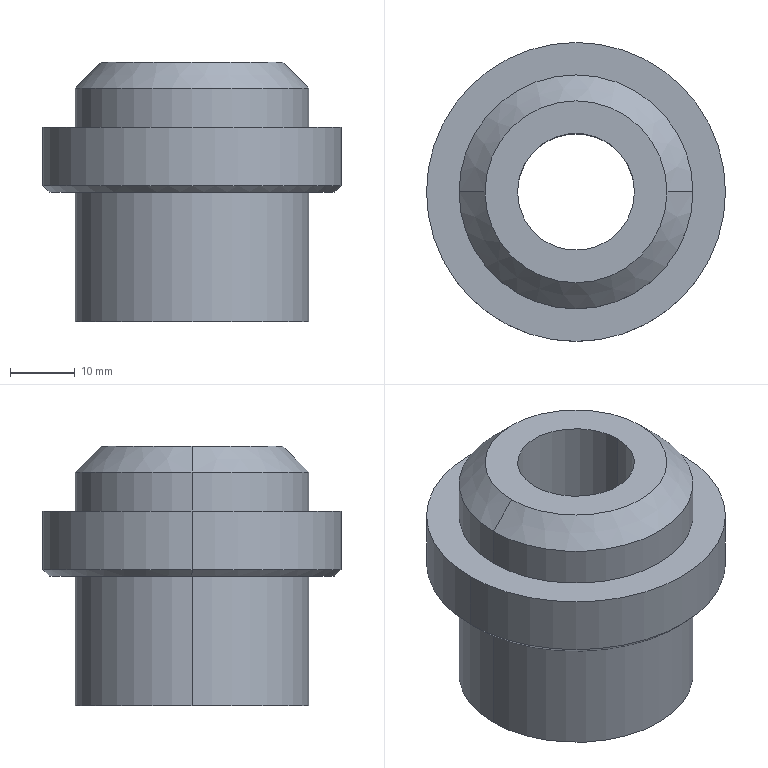Part | SolidWorks | features ICE 3, Chamfer 2, Extrusion 1 | 1 solid | 16 faces | box 46 x 46 x 40 mm | volume 36068 mm3 | cylinder 8 | cone 4 | plane 4 | commonest cylinder face diameters 36 x4 18 x2 46 x2
STEP:
#1=CARTESIAN_POINT('',(-22.,0.,20.));
#2=VERTEX_POINT('',#1);
#3=CARTESIAN_POINT('',(22.,0.,20.));
#4=VERTEX_POINT('',#3);
#5=CARTESIAN_POINT('',(0.,0.,20.));
#6=DIRECTION('',(0.,0.,-1.));
#7=DIRECTION('',(1.,0.,0.));
#8=AXIS2_PLACEMENT_3D('',#5,#6,#7);
#9=CIRCLE('',#8,22.);
#10=EDGE_CURVE('',#2,#4,#9,.T.);
#11=ORIENTED_EDGE('',*,*,#10,.F.);
#12=CARTESIAN_POINT('',(-23.,0.,21.));
#13=VERTEX_POINT('',#12);
#14=CARTESIAN_POINT('',(-23.,0.,21.));
#15=DIRECTION('',(-0.7071,0.,0.7071));
#16=VECTOR('',#15,1000.);
#17=LINE('',#14,#16);
#18=EDGE_CURVE('',#2,#13,#17,.T.);
#19=ORIENTED_EDGE('',*,*,#18,.T.);
#20=CARTESIAN_POINT('',(23.,0.,21.));
#21=VERTEX_POINT('',#20);
#22=CARTESIAN_POINT('',(0.,0.,21.));
#23=DIRECTION('',(0.,0.,1.));
#24=DIRECTION('',(1.,0.,0.));
#25=AXIS2_PLACEMENT_3D('',#22,#23,#24);
#26=CIRCLE('',#25,23.);
#27=EDGE_CURVE('',#21,#13,#26,.T.);
#28=ORIENTED_EDGE('',*,*,#27,.F.);
#29=CARTESIAN_POINT('',(23.,0.,21.));
#30=DIRECTION('',(0.7071,0.,0.7071));
#31=VECTOR('',#30,1000.);
#32=LINE('',#29,#31);
#33=EDGE_CURVE('',#4,#21,#32,.T.);
#34=ORIENTED_EDGE('',*,*,#33,.F.);
#35=EDGE_LOOP('',(#11,#19,#28,#34));
#36=FACE_OUTER_BOUND('',#35,.T.);
#37=CARTESIAN_POINT('',(0.,0.,21.));
#38=DIRECTION('',(0.,0.,1.));
#39=DIRECTION('',(1.,0.,0.));
#40=AXIS2_PLACEMENT_3D('',#37,#38,#39);
#41=CONICAL_SURFACE('',#40,23.,0.7854);
#42=ADVANCED_FACE('',(#36),#41,.T.);
#43=CARTESIAN_POINT('',(-9.,0.,0.));
#44=VERTEX_POINT('',#43);
#45=CARTESIAN_POINT('',(9.,0.,0.));
#46=VERTEX_POINT('',#45);
#47=CARTESIAN_POINT('',(0.,0.,0.));
#48=DIRECTION('',(0.,0.,1.));
#49=DIRECTION('',(1.,0.,0.));
#50=AXIS2_PLACEMENT_3D('',#47,#48,#49);
#51=CIRCLE('',#50,9.);
#52=EDGE_CURVE('',#44,#46,#51,.T.);
#53=ORIENTED_EDGE('',*,*,#52,.F.);
#54=CARTESIAN_POINT('',(-9.,0.,40.));
#55=VERTEX_POINT('',#54);
#56=CARTESIAN_POINT('',(-9.,0.,0.));
#57=DIRECTION('',(0.,0.,1.));
#58=VECTOR('',#57,1000.);
#59=LINE('',#56,#58);
#60=EDGE_CURVE('',#44,#55,#59,.T.);
#61=ORIENTED_EDGE('',*,*,#60,.T.);
#62=CARTESIAN_POINT('',(9.,0.,40.));
#63=VERTEX_POINT('',#62);
#64=CARTESIAN_POINT('',(0.,0.,40.));
#65=DIRECTION('',(0.,0.,1.));
#66=DIRECTION('',(1.,0.,0.));
#67=AXIS2_PLACEMENT_3D('',#64,#65,#66);
#68=CIRCLE('',#67,9.);
#69=EDGE_CURVE('',#55,#63,#68,.T.);
#70=ORIENTED_EDGE('',*,*,#69,.T.);
#71=CARTESIAN_POINT('',(9.,0.,0.));
#72=DIRECTION('',(0.,0.,1.));
#73=VECTOR('',#72,1000.);
#74=LINE('',#71,#73);
#75=EDGE_CURVE('',#46,#63,#74,.T.);
#76=ORIENTED_EDGE('',*,*,#75,.F.);
#77=EDGE_LOOP('',(#53,#61,#70,#76));
#78=FACE_OUTER_BOUND('',#77,.T.);
#79=CARTESIAN_POINT('',(0.,0.,0.));
#80=DIRECTION('',(0.,0.,1.));
#81=DIRECTION('',(1.,0.,0.));
#82=AXIS2_PLACEMENT_3D('',#79,#80,#81);
#83=CYLINDRICAL_SURFACE('',#82,9.);
#84=ADVANCED_FACE('',(#78),#83,.F.);
#85=CARTESIAN_POINT('',(14.,0.,40.));
#86=VERTEX_POINT('',#85);
#87=CARTESIAN_POINT('',(-14.,0.,40.));
#88=VERTEX_POINT('',#87);
#89=CARTESIAN_POINT('',(0.,0.,40.));
#90=DIRECTION('',(0.,0.,1.));
#91=DIRECTION('',(1.,0.,0.));
#92=AXIS2_PLACEMENT_3D('',#89,#90,#91);
#93=CIRCLE('',#92,14.);
#94=EDGE_CURVE('',#86,#88,#93,.T.);
#95=ORIENTED_EDGE('',*,*,#94,.F.);
#96=CARTESIAN_POINT('',(18.,0.,36.));
#97=VERTEX_POINT('',#96);
#98=CARTESIAN_POINT('',(14.,0.,40.));
#99=DIRECTION('',(0.7071,0.,-0.7071));
#100=VECTOR('',#99,1000.);
#101=LINE('',#98,#100);
#102=EDGE_CURVE('',#86,#97,#101,.T.);
#103=ORIENTED_EDGE('',*,*,#102,.T.);
#104=CARTESIAN_POINT('',(-18.,0.,36.));
#105=VERTEX_POINT('',#104);
#106=CARTESIAN_POINT('',(0.,0.,36.));
#107=DIRECTION('',(0.,0.,-1.));
#108=DIRECTION('',(1.,0.,0.));
#109=AXIS2_PLACEMENT_3D('',#106,#107,#108);
#110=CIRCLE('',#109,18.);
#111=EDGE_CURVE('',#105,#97,#110,.T.);
#112=ORIENTED_EDGE('',*,*,#111,.F.);
#113=CARTESIAN_POINT('',(-14.,0.,40.));
#114=DIRECTION('',(-0.7071,0.,-0.7071));
#115=VECTOR('',#114,1000.);
#116=LINE('',#113,#115);
#117=EDGE_CURVE('',#88,#105,#116,.T.);
#118=ORIENTED_EDGE('',*,*,#117,.F.);
#119=EDGE_LOOP('',(#95,#103,#112,#118));
#120=FACE_OUTER_BOUND('',#119,.T.);
#121=CARTESIAN_POINT('',(0.,0.,40.));
#122=DIRECTION('',(0.,0.,-1.));
#123=DIRECTION('',(-1.,0.,0.));
#124=AXIS2_PLACEMENT_3D('',#121,#122,#123);
#125=CONICAL_SURFACE('',#124,14.,0.7854);
#126=ADVANCED_FACE('',(#120),#125,.T.);
#127=ORIENTED_EDGE('',*,*,#111,.T.);
#128=CARTESIAN_POINT('',(18.,0.,30.));
#129=VERTEX_POINT('',#128);
#130=CARTESIAN_POINT('',(18.,0.,40.));
#131=DIRECTION('',(0.,0.,-1.));
#132=VECTOR('',#131,1000.);
#133=LINE('',#130,#132);
#134=EDGE_CURVE('',#97,#129,#133,.T.);
#135=ORIENTED_EDGE('',*,*,#134,.T.);
#136=CARTESIAN_POINT('',(-18.,0.,30.));
#137=VERTEX_POINT('',#136);
#138=CARTESIAN_POINT('',(0.,0.,30.));
#139=DIRECTION('',(0.,0.,1.));
#140=DIRECTION('',(1.,0.,0.));
#141=AXIS2_PLACEMENT_3D('',#138,#139,#140);
#142=CIRCLE('',#141,18.);
#143=EDGE_CURVE('',#129,#137,#142,.T.);
#144=ORIENTED_EDGE('',*,*,#143,.T.);
#145=CARTESIAN_POINT('',(-18.,0.,40.));
#146=DIRECTION('',(0.,0.,-1.));
#147=VECTOR('',#146,1000.);
#148=LINE('',#145,#147);
#149=EDGE_CURVE('',#105,#137,#148,.T.);
#150=ORIENTED_EDGE('',*,*,#149,.F.);
#151=EDGE_LOOP('',(#127,#135,#144,#150));
#152=FACE_OUTER_BOUND('',#151,.T.);
#153=CARTESIAN_POINT('',(0.,0.,40.));
#154=DIRECTION('',(0.,0.,-1.));
#155=DIRECTION('',(-1.,0.,0.));
#156=AXIS2_PLACEMENT_3D('',#153,#154,#155);
#157=CYLINDRICAL_SURFACE('',#156,18.);
#158=ADVANCED_FACE('',(#152),#157,.T.);
#159=CARTESIAN_POINT('',(23.,0.,30.));
#160=VERTEX_POINT('',#159);
#161=CARTESIAN_POINT('',(-23.,0.,30.));
#162=VERTEX_POINT('',#161);
#163=CARTESIAN_POINT('',(0.,0.,30.));
#164=DIRECTION('',(0.,0.,1.));
#165=DIRECTION('',(1.,0.,0.));
#166=AXIS2_PLACEMENT_3D('',#163,#164,#165);
#167=CIRCLE('',#166,23.);
#168=EDGE_CURVE('',#160,#162,#167,.T.);
#169=ORIENTED_EDGE('',*,*,#168,.F.);
#170=CARTESIAN_POINT('',(23.,0.,30.));
#171=DIRECTION('',(0.,0.,-1.));
#172=VECTOR('',#171,1000.);
#173=LINE('',#170,#172);
#174=EDGE_CURVE('',#160,#21,#173,.T.);
#175=ORIENTED_EDGE('',*,*,#174,.T.);
#176=ORIENTED_EDGE('',*,*,#27,.T.);
#177=CARTESIAN_POINT('',(-23.,0.,30.));
#178=DIRECTION('',(0.,0.,-1.));
#179=VECTOR('',#178,1000.);
#180=LINE('',#177,#179);
#181=EDGE_CURVE('',#162,#13,#180,.T.);
#182=ORIENTED_EDGE('',*,*,#181,.F.);
#183=EDGE_LOOP('',(#169,#175,#176,#182));
#184=FACE_OUTER_BOUND('',#183,.T.);
#185=CARTESIAN_POINT('',(0.,0.,30.));
#186=DIRECTION('',(0.,0.,-1.));
#187=DIRECTION('',(-1.,0.,0.));
#188=AXIS2_PLACEMENT_3D('',#185,#186,#187);
#189=CYLINDRICAL_SURFACE('',#188,23.);
#190=ADVANCED_FACE('',(#184),#189,.T.);
#191=CARTESIAN_POINT('',(18.,0.,20.));
#192=VERTEX_POINT('',#191);
#193=CARTESIAN_POINT('',(-18.,0.,20.));
#194=VERTEX_POINT('',#193);
#195=CARTESIAN_POINT('',(0.,0.,20.));
#196=DIRECTION('',(0.,0.,1.));
#197=DIRECTION('',(1.,0.,0.));
#198=AXIS2_PLACEMENT_3D('',#195,#196,#197);
#199=CIRCLE('',#198,18.);
#200=EDGE_CURVE('',#192,#194,#199,.T.);
#201=ORIENTED_EDGE('',*,*,#200,.F.);
#202=CARTESIAN_POINT('',(18.,0.,0.));
#203=VERTEX_POINT('',#202);
#204=CARTESIAN_POINT('',(18.,0.,20.));
#205=DIRECTION('',(0.,0.,-1.));
#206=VECTOR('',#205,1000.);
#207=LINE('',#204,#206);
#208=EDGE_CURVE('',#192,#203,#207,.T.);
#209=ORIENTED_EDGE('',*,*,#208,.T.);
#210=CARTESIAN_POINT('',(-18.,0.,0.));
#211=VERTEX_POINT('',#210);
#212=CARTESIAN_POINT('',(0.,0.,0.));
#213=DIRECTION('',(0.,0.,1.));
#214=DIRECTION('',(1.,0.,0.));
#215=AXIS2_PLACEMENT_3D('',#212,#213,#214);
#216=CIRCLE('',#215,18.);
#217=EDGE_CURVE('',#203,#211,#216,.T.);
#218=ORIENTED_EDGE('',*,*,#217,.T.);
#219=CARTESIAN_POINT('',(-18.,0.,20.));
#220=DIRECTION('',(0.,0.,-1.));
#221=VECTOR('',#220,1000.);
#222=LINE('',#219,#221);
#223=EDGE_CURVE('',#194,#211,#222,.T.);
#224=ORIENTED_EDGE('',*,*,#223,.F.);
#225=EDGE_LOOP('',(#201,#209,#218,#224));
#226=FACE_OUTER_BOUND('',#225,.T.);
#227=CARTESIAN_POINT('',(0.,0.,20.));
#228=DIRECTION('',(0.,0.,-1.));
#229=DIRECTION('',(-1.,0.,0.));
#230=AXIS2_PLACEMENT_3D('',#227,#228,#229);
#231=CYLINDRICAL_SURFACE('',#230,18.);
#232=ADVANCED_FACE('',(#226),#231,.T.);
#233=ORIENTED_EDGE('',*,*,#208,.F.);
#234=CARTESIAN_POINT('',(0.,0.,20.));
#235=DIRECTION('',(0.,0.,1.));
#236=DIRECTION('',(1.,0.,0.));
#237=AXIS2_PLACEMENT_3D('',#234,#235,#236);
#238=CIRCLE('',#237,18.);
#239=EDGE_CURVE('',#194,#192,#238,.T.);
#240=ORIENTED_EDGE('',*,*,#239,.F.);
#241=ORIENTED_EDGE('',*,*,#223,.T.);
#242=CARTESIAN_POINT('',(0.,0.,0.));
#243=DIRECTION('',(0.,0.,1.));
#244=DIRECTION('',(1.,0.,0.));
#245=AXIS2_PLACEMENT_3D('',#242,#243,#244);
#246=CIRCLE('',#245,18.);
#247=EDGE_CURVE('',#211,#203,#246,.T.);
#248=ORIENTED_EDGE('',*,*,#247,.T.);
#249=EDGE_LOOP('',(#233,#240,#241,#248));
#250=FACE_OUTER_BOUND('',#249,.T.);
#251=CARTESIAN_POINT('',(0.,0.,20.));
#252=DIRECTION('',(0.,0.,-1.));
#253=DIRECTION('',(-1.,0.,0.));
#254=AXIS2_PLACEMENT_3D('',#251,#252,#253);
#255=CYLINDRICAL_SURFACE('',#254,18.);
#256=ADVANCED_FACE('',(#250),#255,.T.);
#257=CARTESIAN_POINT('',(0.,0.,0.));
#258=DIRECTION('',(0.,0.,1.));
#259=DIRECTION('',(1.,0.,0.));
#260=AXIS2_PLACEMENT_3D('',#257,#258,#259);
#261=CIRCLE('',#260,9.);
#262=EDGE_CURVE('',#46,#44,#261,.T.);
#263=ORIENTED_EDGE('',*,*,#262,.T.);
#264=ORIENTED_EDGE('',*,*,#52,.T.);
#265=EDGE_LOOP('',(#263,#264));
#266=FACE_BOUND('',#265,.T.);
#267=ORIENTED_EDGE('',*,*,#247,.F.);
#268=ORIENTED_EDGE('',*,*,#217,.F.);
#269=EDGE_LOOP('',(#267,#268));
#270=FACE_OUTER_BOUND('',#269,.T.);
#271=CARTESIAN_POINT('',(0.,0.,0.));
#272=DIRECTION('',(0.,0.,1.));
#273=DIRECTION('',(1.,0.,0.));
#274=AXIS2_PLACEMENT_3D('',#271,#272,#273);
#275=PLANE('',#274);
#276=ADVANCED_FACE('',(#266,#270),#275,.F.);
#277=ORIENTED_EDGE('',*,*,#174,.F.);
#278=CARTESIAN_POINT('',(0.,0.,30.));
#279=DIRECTION('',(0.,0.,1.));
#280=DIRECTION('',(1.,0.,0.));
#281=AXIS2_PLACEMENT_3D('',#278,#279,#280);
#282=CIRCLE('',#281,23.);
#283=EDGE_CURVE('',#162,#160,#282,.T.);
#284=ORIENTED_EDGE('',*,*,#283,.F.);
#285=ORIENTED_EDGE('',*,*,#181,.T.);
#286=CARTESIAN_POINT('',(0.,0.,21.));
#287=DIRECTION('',(0.,0.,1.));
#288=DIRECTION('',(1.,0.,0.));
#289=AXIS2_PLACEMENT_3D('',#286,#287,#288);
#290=CIRCLE('',#289,23.);
#291=EDGE_CURVE('',#13,#21,#290,.T.);
#292=ORIENTED_EDGE('',*,*,#291,.T.);
#293=EDGE_LOOP('',(#277,#284,#285,#292));
#294=FACE_OUTER_BOUND('',#293,.T.);
#295=CARTESIAN_POINT('',(0.,0.,30.));
#296=DIRECTION('',(0.,0.,-1.));
#297=DIRECTION('',(-1.,0.,0.));
#298=AXIS2_PLACEMENT_3D('',#295,#296,#297);
#299=CYLINDRICAL_SURFACE('',#298,23.);
#300=ADVANCED_FACE('',(#294),#299,.T.);
#301=CARTESIAN_POINT('',(0.,0.,30.));
#302=DIRECTION('',(0.,0.,1.));
#303=DIRECTION('',(1.,0.,0.));
#304=AXIS2_PLACEMENT_3D('',#301,#302,#303);
#305=CIRCLE('',#304,18.);
#306=EDGE_CURVE('',#137,#129,#305,.T.);
#307=ORIENTED_EDGE('',*,*,#306,.F.);
#308=ORIENTED_EDGE('',*,*,#143,.F.);
#309=EDGE_LOOP('',(#307,#308));
#310=FACE_BOUND('',#309,.T.);
#311=ORIENTED_EDGE('',*,*,#283,.T.);
#312=ORIENTED_EDGE('',*,*,#168,.T.);
#313=EDGE_LOOP('',(#311,#312));
#314=FACE_OUTER_BOUND('',#313,.T.);
#315=CARTESIAN_POINT('',(0.,0.,30.));
#316=DIRECTION('',(0.,0.,1.));
#317=DIRECTION('',(1.,0.,0.));
#318=AXIS2_PLACEMENT_3D('',#315,#316,#317);
#319=PLANE('',#318);
#320=ADVANCED_FACE('',(#310,#314),#319,.T.);
#321=CARTESIAN_POINT('',(0.,0.,20.));
#322=DIRECTION('',(0.,0.,-1.));
#323=DIRECTION('',(1.,0.,0.));
#324=AXIS2_PLACEMENT_3D('',#321,#322,#323);
#325=CIRCLE('',#324,22.);
#326=EDGE_CURVE('',#4,#2,#325,.T.);
#327=ORIENTED_EDGE('',*,*,#326,.T.);
#328=ORIENTED_EDGE('',*,*,#10,.T.);
#329=EDGE_LOOP('',(#327,#328));
#330=FACE_OUTER_BOUND('',#329,.T.);
#331=ORIENTED_EDGE('',*,*,#239,.T.);
#332=ORIENTED_EDGE('',*,*,#200,.T.);
#333=EDGE_LOOP('',(#331,#332));
#334=FACE_BOUND('',#333,.T.);
#335=CARTESIAN_POINT('',(0.,0.,20.));
#336=DIRECTION('',(0.,0.,1.));
#337=DIRECTION('',(1.,0.,0.));
#338=AXIS2_PLACEMENT_3D('',#335,#336,#337);
#339=PLANE('',#338);
#340=ADVANCED_FACE('',(#330,#334),#339,.F.);
#341=ORIENTED_EDGE('',*,*,#134,.F.);
#342=CARTESIAN_POINT('',(0.,0.,36.));
#343=DIRECTION('',(0.,0.,-1.));
#344=DIRECTION('',(1.,0.,0.));
#345=AXIS2_PLACEMENT_3D('',#342,#343,#344);
#346=CIRCLE('',#345,18.);
#347=EDGE_CURVE('',#97,#105,#346,.T.);
#348=ORIENTED_EDGE('',*,*,#347,.T.);
#349=ORIENTED_EDGE('',*,*,#149,.T.);
#350=ORIENTED_EDGE('',*,*,#306,.T.);
#351=EDGE_LOOP('',(#341,#348,#349,#350));
#352=FACE_OUTER_BOUND('',#351,.T.);
#353=CARTESIAN_POINT('',(0.,0.,40.));
#354=DIRECTION('',(0.,0.,-1.));
#355=DIRECTION('',(-1.,0.,0.));
#356=AXIS2_PLACEMENT_3D('',#353,#354,#355);
#357=CYLINDRICAL_SURFACE('',#356,18.);
#358=ADVANCED_FACE('',(#352),#357,.T.);
#359=CARTESIAN_POINT('',(0.,0.,40.));
#360=DIRECTION('',(0.,0.,1.));
#361=DIRECTION('',(1.,0.,0.));
#362=AXIS2_PLACEMENT_3D('',#359,#360,#361);
#363=CIRCLE('',#362,9.);
#364=EDGE_CURVE('',#63,#55,#363,.T.);
#365=ORIENTED_EDGE('',*,*,#364,.F.);
#366=ORIENTED_EDGE('',*,*,#69,.F.);
#367=EDGE_LOOP('',(#365,#366));
#368=FACE_BOUND('',#367,.T.);
#369=CARTESIAN_POINT('',(0.,0.,40.));
#370=DIRECTION('',(0.,0.,1.));
#371=DIRECTION('',(1.,0.,0.));
#372=AXIS2_PLACEMENT_3D('',#369,#370,#371);
#373=CIRCLE('',#372,14.);
#374=EDGE_CURVE('',#88,#86,#373,.T.);
#375=ORIENTED_EDGE('',*,*,#374,.T.);
#376=ORIENTED_EDGE('',*,*,#94,.T.);
#377=EDGE_LOOP('',(#375,#376));
#378=FACE_OUTER_BOUND('',#377,.T.);
#379=CARTESIAN_POINT('',(0.,0.,40.));
#380=DIRECTION('',(0.,0.,1.));
#381=DIRECTION('',(1.,0.,0.));
#382=AXIS2_PLACEMENT_3D('',#379,#380,#381);
#383=PLANE('',#382);
#384=ADVANCED_FACE('',(#368,#378),#383,.T.);
#385=ORIENTED_EDGE('',*,*,#102,.F.);
#386=ORIENTED_EDGE('',*,*,#374,.F.);
#387=ORIENTED_EDGE('',*,*,#117,.T.);
#388=ORIENTED_EDGE('',*,*,#347,.F.);
#389=EDGE_LOOP('',(#385,#386,#387,#388));
#390=FACE_OUTER_BOUND('',#389,.T.);
#391=CARTESIAN_POINT('',(0.,0.,40.));
#392=DIRECTION('',(0.,0.,-1.));
#393=DIRECTION('',(-1.,0.,0.));
#394=AXIS2_PLACEMENT_3D('',#391,#392,#393);
#395=CONICAL_SURFACE('',#394,14.,0.7854);
#396=ADVANCED_FACE('',(#390),#395,.T.);
#397=ORIENTED_EDGE('',*,*,#60,.F.);
#398=ORIENTED_EDGE('',*,*,#262,.F.);
#399=ORIENTED_EDGE('',*,*,#75,.T.);
#400=ORIENTED_EDGE('',*,*,#364,.T.);
#401=EDGE_LOOP('',(#397,#398,#399,#400));
#402=FACE_OUTER_BOUND('',#401,.T.);
#403=CARTESIAN_POINT('',(0.,0.,0.));
#404=DIRECTION('',(0.,0.,1.));
#405=DIRECTION('',(1.,0.,0.));
#406=AXIS2_PLACEMENT_3D('',#403,#404,#405);
#407=CYLINDRICAL_SURFACE('',#406,9.);
#408=ADVANCED_FACE('',(#402),#407,.F.);
#409=ORIENTED_EDGE('',*,*,#18,.F.);
#410=ORIENTED_EDGE('',*,*,#326,.F.);
#411=ORIENTED_EDGE('',*,*,#33,.T.);
#412=ORIENTED_EDGE('',*,*,#291,.F.);
#413=EDGE_LOOP('',(#409,#410,#411,#412));
#414=FACE_OUTER_BOUND('',#413,.T.);
#415=CARTESIAN_POINT('',(0.,0.,21.));
#416=DIRECTION('',(0.,0.,1.));
#417=DIRECTION('',(1.,0.,0.));
#418=AXIS2_PLACEMENT_3D('',#415,#416,#417);
#419=CONICAL_SURFACE('',#418,23.,0.7854);
#420=ADVANCED_FACE('',(#414),#419,.T.);
#421=CLOSED_SHELL('',(#42,#84,#126,#158,#190,#232,#256,#276,#300,#320,#340,#358,#384,#396,#408,#420));
#422=MANIFOLD_SOLID_BREP('',#421);
#423=CARTESIAN_POINT('',(0.,0.,0.));
#424=DIRECTION('',(0.,0.,1.));
#425=DIRECTION('',(1.,0.,0.));
#426=AXIS2_PLACEMENT_3D('',#423,#424,#425);
#427=(LENGTH_UNIT()NAMED_UNIT(*)SI_UNIT(.MILLI.,.METRE.));
#428=UNCERTAINTY_MEASURE_WITH_UNIT(LENGTH_MEASURE(0.00001),#427,'','');
#429=(NAMED_UNIT(*)PLANE_ANGLE_UNIT()SI_UNIT($,.RADIAN.));
#430=(NAMED_UNIT(*)SI_UNIT($,.STERADIAN.)SOLID_ANGLE_UNIT());
#431=(GEOMETRIC_REPRESENTATION_CONTEXT(3)GLOBAL_UNCERTAINTY_ASSIGNED_CONTEXT((#428))GLOBAL_UNIT_ASSIGNED_CONTEXT((#427,#429,#430))REPRESENTATION_CONTEXT('',''));
#432=ADVANCED_BREP_SHAPE_REPRESENTATION('',(#422,#426),#431);